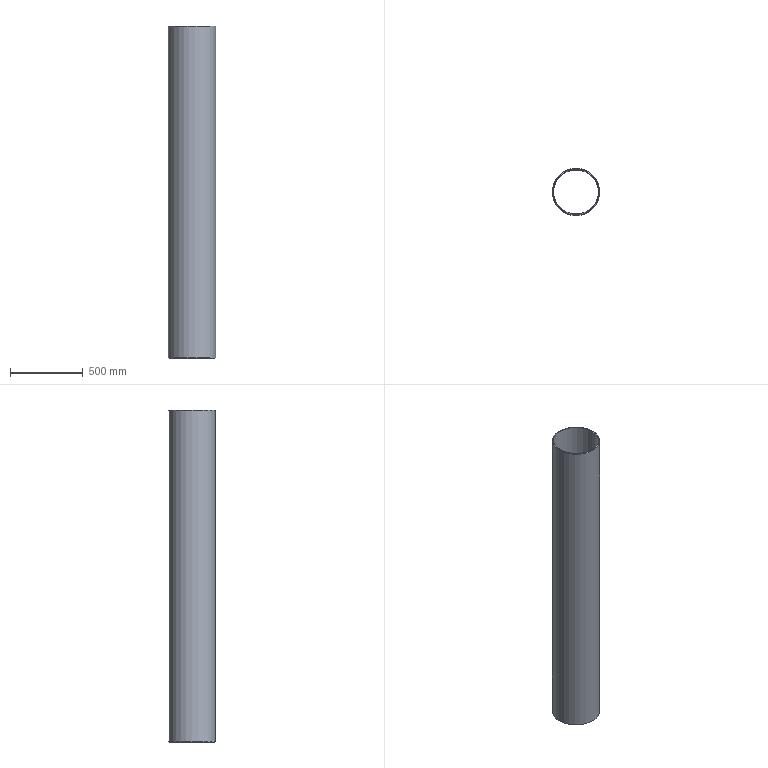Part | NX | features CHAMFER 1, CYLINDER 1, DATUM_CSYS 1, SHELL 1 | 1 solid | 6 faces | box 325 x 325 x 2289 mm | volume 18225689 mm3 | plane 2 | cylinder 2 | cone 2 | commonest cylinder face diameters 309 x1 325 x1
STEP:
#1=CARTESIAN_POINT('',(158.17,0.,2289.));
#2=VERTEX_POINT('',#1);
#3=CARTESIAN_POINT('',(0.,0.,2289.));
#4=DIRECTION('',(0.,0.,1.));
#5=DIRECTION('',(1.,0.,0.));
#6=AXIS2_PLACEMENT_3D('',#3,#4,#5);
#7=CIRCLE('',#6,158.17);
#8=EDGE_CURVE('',#2,#2,#7,.T.);
#9=ORIENTED_EDGE('',*,*,#8,.T.);
#10=EDGE_LOOP('',(#9));
#11=FACE_BOUND('',#10,.T.);
#12=CARTESIAN_POINT('',(154.5,0.,2289.));
#13=VERTEX_POINT('',#12);
#14=CARTESIAN_POINT('',(0.,0.,2289.));
#15=DIRECTION('',(0.,0.,1.));
#16=DIRECTION('',(1.,0.,0.));
#17=AXIS2_PLACEMENT_3D('',#14,#15,#16);
#18=CIRCLE('',#17,154.5);
#19=EDGE_CURVE('',#13,#13,#18,.F.);
#20=ORIENTED_EDGE('',*,*,#19,.T.);
#21=EDGE_LOOP('',(#20));
#22=FACE_BOUND('',#21,.T.);
#23=CARTESIAN_POINT('',(0.,0.,2289.));
#24=DIRECTION('',(0.,0.,1.));
#25=DIRECTION('',(1.,0.,0.));
#26=AXIS2_PLACEMENT_3D('',#23,#24,#25);
#27=PLANE('',#26);
#28=ADVANCED_FACE('',(#11,#22),#27,.T.);
#29=CARTESIAN_POINT('',(-158.17,0.,0.));
#30=VERTEX_POINT('',#29);
#31=CARTESIAN_POINT('',(0.,0.,0.));
#32=DIRECTION('',(0.,0.,-1.));
#33=DIRECTION('',(-1.,0.,0.));
#34=AXIS2_PLACEMENT_3D('',#31,#32,#33);
#35=CIRCLE('',#34,158.17);
#36=EDGE_CURVE('',#30,#30,#35,.T.);
#37=ORIENTED_EDGE('',*,*,#36,.T.);
#38=EDGE_LOOP('',(#37));
#39=FACE_BOUND('',#38,.T.);
#40=CARTESIAN_POINT('',(-154.5,0.,0.));
#41=VERTEX_POINT('',#40);
#42=CARTESIAN_POINT('',(0.,0.,0.));
#43=DIRECTION('',(0.,0.,-1.));
#44=DIRECTION('',(-1.,0.,0.));
#45=AXIS2_PLACEMENT_3D('',#42,#43,#44);
#46=CIRCLE('',#45,154.5);
#47=EDGE_CURVE('',#41,#41,#46,.F.);
#48=ORIENTED_EDGE('',*,*,#47,.T.);
#49=EDGE_LOOP('',(#48));
#50=FACE_BOUND('',#49,.T.);
#51=CARTESIAN_POINT('',(0.,0.,0.));
#52=DIRECTION('',(0.,0.,-1.));
#53=DIRECTION('',(-1.,0.,0.));
#54=AXIS2_PLACEMENT_3D('',#51,#52,#53);
#55=PLANE('',#54);
#56=ADVANCED_FACE('',(#39,#50),#55,.T.);
#57=CARTESIAN_POINT('',(-162.5,0.,2.5));
#58=VERTEX_POINT('',#57);
#59=CARTESIAN_POINT('',(0.,0.,2.5));
#60=DIRECTION('',(0.,0.,-1.));
#61=DIRECTION('',(-1.,0.,0.));
#62=AXIS2_PLACEMENT_3D('',#59,#60,#61);
#63=CIRCLE('',#62,162.5);
#64=EDGE_CURVE('',#58,#58,#63,.F.);
#65=ORIENTED_EDGE('',*,*,#64,.T.);
#66=EDGE_LOOP('',(#65));
#67=FACE_BOUND('',#66,.T.);
#68=CARTESIAN_POINT('',(162.5,0.,2286.5));
#69=VERTEX_POINT('',#68);
#70=CARTESIAN_POINT('',(0.,0.,2286.5));
#71=DIRECTION('',(0.,0.,1.));
#72=DIRECTION('',(1.,0.,0.));
#73=AXIS2_PLACEMENT_3D('',#70,#71,#72);
#74=CIRCLE('',#73,162.5);
#75=EDGE_CURVE('',#69,#69,#74,.F.);
#76=ORIENTED_EDGE('',*,*,#75,.T.);
#77=EDGE_LOOP('',(#76));
#78=FACE_BOUND('',#77,.T.);
#79=CARTESIAN_POINT('',(0.,0.,0.));
#80=DIRECTION('',(0.,0.,1.));
#81=DIRECTION('',(1.,0.,0.));
#82=AXIS2_PLACEMENT_3D('',#79,#80,#81);
#83=CYLINDRICAL_SURFACE('',#82,162.5);
#84=ADVANCED_FACE('',(#67,#78),#83,.T.);
#85=ORIENTED_EDGE('',*,*,#19,.F.);
#86=EDGE_LOOP('',(#85));
#87=FACE_BOUND('',#86,.T.);
#88=ORIENTED_EDGE('',*,*,#47,.F.);
#89=EDGE_LOOP('',(#88));
#90=FACE_BOUND('',#89,.T.);
#91=CARTESIAN_POINT('',(0.,0.,0.));
#92=DIRECTION('',(0.,0.,1.));
#93=DIRECTION('',(1.,0.,0.));
#94=AXIS2_PLACEMENT_3D('',#91,#92,#93);
#95=CYLINDRICAL_SURFACE('',#94,154.5);
#96=ADVANCED_FACE('',(#87,#90),#95,.F.);
#97=ORIENTED_EDGE('',*,*,#36,.F.);
#98=EDGE_LOOP('',(#97));
#99=FACE_BOUND('',#98,.T.);
#100=ORIENTED_EDGE('',*,*,#64,.F.);
#101=EDGE_LOOP('',(#100));
#102=FACE_BOUND('',#101,.T.);
#103=CARTESIAN_POINT('',(0.,0.,2.5));
#104=DIRECTION('',(0.,0.,1.));
#105=DIRECTION('',(1.,0.,0.));
#106=AXIS2_PLACEMENT_3D('',#103,#104,#105);
#107=CONICAL_SURFACE('',#106,162.5,1.047);
#108=ADVANCED_FACE('',(#99,#102),#107,.T.);
#109=ORIENTED_EDGE('',*,*,#8,.F.);
#110=EDGE_LOOP('',(#109));
#111=FACE_BOUND('',#110,.T.);
#112=ORIENTED_EDGE('',*,*,#75,.F.);
#113=EDGE_LOOP('',(#112));
#114=FACE_BOUND('',#113,.T.);
#115=CARTESIAN_POINT('',(0.,0.,2286.5));
#116=DIRECTION('',(0.,0.,-1.));
#117=DIRECTION('',(-1.,0.,0.));
#118=AXIS2_PLACEMENT_3D('',#115,#116,#117);
#119=CONICAL_SURFACE('',#118,162.5,1.047);
#120=ADVANCED_FACE('',(#111,#114),#119,.T.);
#121=CLOSED_SHELL('',(#28,#56,#84,#96,#108,#120));
#122=MANIFOLD_SOLID_BREP('',#121);
#123=(LENGTH_UNIT()NAMED_UNIT(*)SI_UNIT(.MILLI.,.METRE.));
#124=UNCERTAINTY_MEASURE_WITH_UNIT(LENGTH_MEASURE(0.00001),#123,'','');
#125=(NAMED_UNIT(*)PLANE_ANGLE_UNIT()SI_UNIT($,.RADIAN.));
#126=(NAMED_UNIT(*)SI_UNIT($,.STERADIAN.)SOLID_ANGLE_UNIT());
#127=(GEOMETRIC_REPRESENTATION_CONTEXT(3)GLOBAL_UNCERTAINTY_ASSIGNED_CONTEXT((#124))GLOBAL_UNIT_ASSIGNED_CONTEXT((#123,#125,#126))REPRESENTATION_CONTEXT('',''));
#128=ADVANCED_BREP_SHAPE_REPRESENTATION('',(#122),#127);